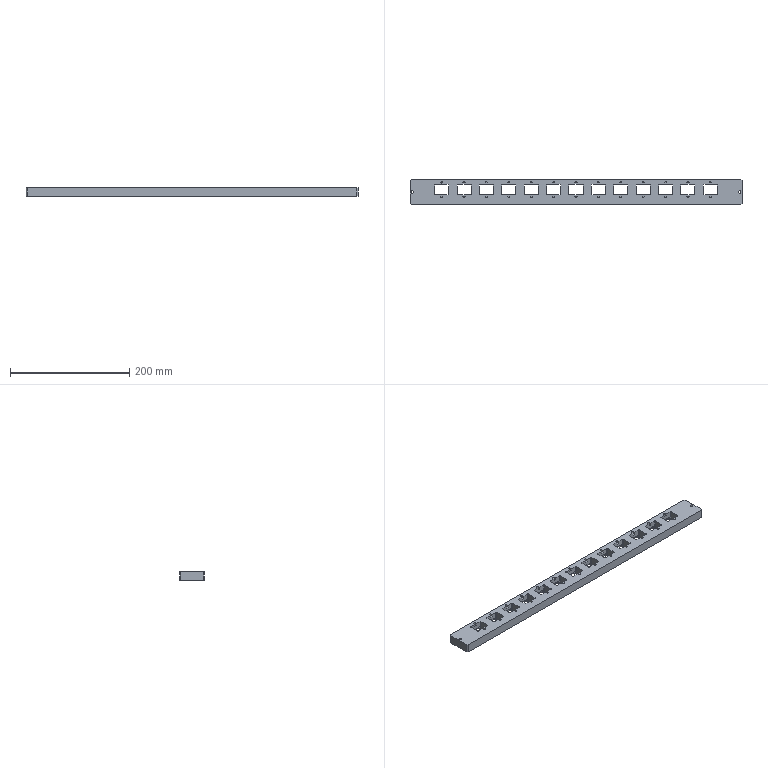Part | 1 solid | 432 faces | box 556 x 41 x 15 mm | volume 253236 mm3 | plane 272 | cylinder 160 | commonest cylinder face diameters 2 x156 0.3 x2 4 x2